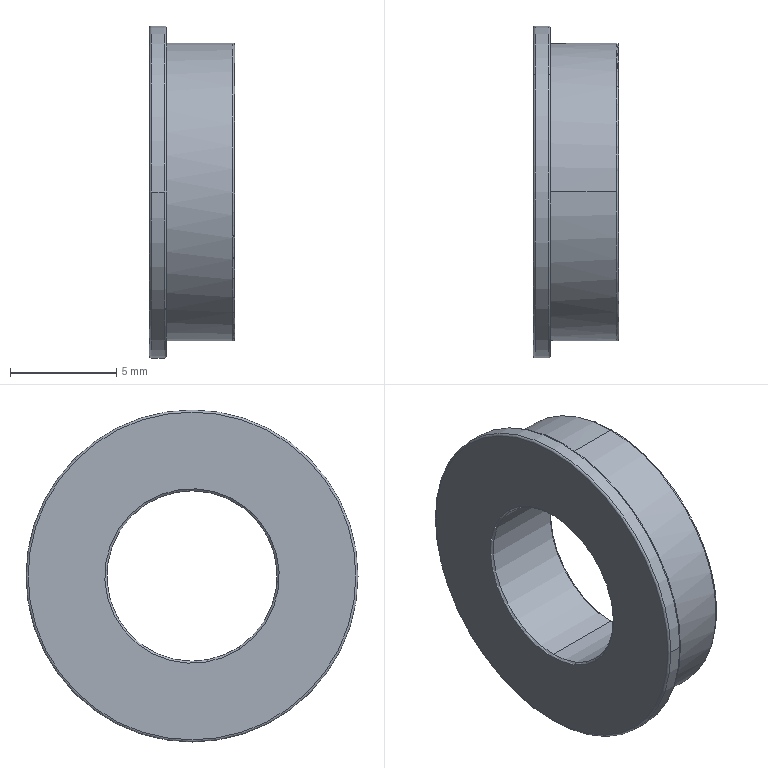Part | STEP file | ASND-0110-0502110051 | 1 solid | 19 faces | box 4 x 15.6 x 15.6 mm | volume 444.035 mm3 | torus 10 | cylinder 6 | plane 3 | commonest cylinder face diameters 8 x2 14 x2 15.6 x2
STEP:
#1=CARTESIAN_POINT('',(0.,0.,0.));
#2=DIRECTION('',(0.,0.,1.));
#3=DIRECTION('',(1.,0.,0.));
#4=AXIS2_PLACEMENT_3D('',#1,#2,#3);
#5=CARTESIAN_POINT('',(0.,-5.445,-5.445));
#6=VERTEX_POINT('',#5);
#7=CARTESIAN_POINT('',(0.,5.445,5.445));
#8=VERTEX_POINT('',#7);
#9=CARTESIAN_POINT('',(0.,0.,0.));
#10=DIRECTION('',(-1.,0.,0.));
#11=DIRECTION('',(0.,1.,0.));
#12=AXIS2_PLACEMENT_3D('',#9,#10,#11);
#13=CIRCLE('',#12,7.7);
#14=CARTESIAN_POINT('',(0.1,0.,0.));
#15=DIRECTION('',(1.,0.,0.));
#16=DIRECTION('',(0.,0.7071,0.7071));
#17=AXIS2_PLACEMENT_3D('',#14,#15,#16);
#18=TOROIDAL_SURFACE('',#17,7.7,0.1);
#19=CARTESIAN_POINT('',(5.498,4.712));
#20=DIRECTION('',(-1.,0.));
#21=VECTOR('',#20,1.);
#22=LINE('',#19,#21);
#23=(GEOMETRIC_REPRESENTATION_CONTEXT(2)PARAMETRIC_REPRESENTATION_CONTEXT()REPRESENTATION_CONTEXT('',''));
#24=DEFINITIONAL_REPRESENTATION('',(#22),#23);
#25=PCURVE('',#18,#24);
#26=CARTESIAN_POINT('',(0.,0.,0.));
#27=DIRECTION('',(1.,0.,0.));
#28=DIRECTION('',(0.,0.7071,0.7071));
#29=AXIS2_PLACEMENT_3D('',#26,#27,#28);
#30=PLANE('',#29);
#31=CARTESIAN_POINT('',(5.445,-5.445));
#32=CARTESIAN_POINT('',(-3.986,-14.875));
#33=CARTESIAN_POINT('',(-7.438,-1.993));
#34=CARTESIAN_POINT('',(-10.889,10.889));
#35=CARTESIAN_POINT('',(1.993,7.438));
#36=CARTESIAN_POINT('',(14.875,3.986));
#37=CARTESIAN_POINT('',(5.445,-5.445));
#38=(BOUNDED_CURVE()B_SPLINE_CURVE(2,(#31,#32,#33,#34,#35,#36,#37),.UNSPECIFIED.,.T.,.F.)B_SPLINE_CURVE_WITH_KNOTS((1,2,2,2,2,1),(-2.094,0.,2.094,4.189,6.283,8.378),.UNSPECIFIED.)CURVE()GEOMETRIC_REPRESENTATION_ITEM()RATIONAL_B_SPLINE_CURVE((1.,0.5,1.,0.5,1.,0.5,1.))REPRESENTATION_ITEM(''));
#39=(GEOMETRIC_REPRESENTATION_CONTEXT(2)PARAMETRIC_REPRESENTATION_CONTEXT()REPRESENTATION_CONTEXT('',''));
#40=DEFINITIONAL_REPRESENTATION('',(#38),#39);
#41=PCURVE('',#30,#40);
#42=SURFACE_CURVE('',#13,(#25,#41),.PCURVE_S1.);
#43=EDGE_CURVE('',#6,#8,#42,.T.);
#44=ORIENTED_EDGE('',*,*,#43,.F.);
#45=CARTESIAN_POINT('',(0.1,-5.515,-5.515));
#46=VERTEX_POINT('',#45);
#47=CARTESIAN_POINT('',(0.1,-5.445,-5.445));
#48=DIRECTION('',(0.,-0.7071,0.7071));
#49=DIRECTION('',(0.,-0.7071,-0.7071));
#50=AXIS2_PLACEMENT_3D('',#47,#48,#49);
#51=CIRCLE('',#50,0.1);
#52=CARTESIAN_POINT('',(3.142,0.));
#53=DIRECTION('',(0.,1.));
#54=VECTOR('',#53,1.);
#55=LINE('',#52,#54);
#56=(GEOMETRIC_REPRESENTATION_CONTEXT(2)PARAMETRIC_REPRESENTATION_CONTEXT()REPRESENTATION_CONTEXT('',''));
#57=DEFINITIONAL_REPRESENTATION('',(#55),#56);
#58=PCURVE('',#18,#57);
#59=CARTESIAN_POINT('',(0.1,0.,0.));
#60=DIRECTION('',(1.,0.,0.));
#61=DIRECTION('',(0.,0.7071,0.7071));
#62=AXIS2_PLACEMENT_3D('',#59,#60,#61);
#63=TOROIDAL_SURFACE('',#62,7.7,0.1);
#64=CARTESIAN_POINT('',(3.142,0.));
#65=DIRECTION('',(0.,1.));
#66=VECTOR('',#65,1.);
#67=LINE('',#64,#66);
#68=(GEOMETRIC_REPRESENTATION_CONTEXT(2)PARAMETRIC_REPRESENTATION_CONTEXT()REPRESENTATION_CONTEXT('',''));
#69=DEFINITIONAL_REPRESENTATION('',(#67),#68);
#70=PCURVE('',#63,#69);
#71=SURFACE_CURVE('',#51,(#58,#70),.PCURVE_S1.);
#72=EDGE_CURVE('',#6,#46,#71,.T.);
#73=ORIENTED_EDGE('',*,*,#72,.T.);
#74=CARTESIAN_POINT('',(0.1,-7.8,0.));
#75=VERTEX_POINT('',#74);
#76=CARTESIAN_POINT('',(0.1,0.,0.));
#77=DIRECTION('',(-1.,0.,0.));
#78=DIRECTION('',(0.,1.,0.));
#79=AXIS2_PLACEMENT_3D('',#76,#77,#78);
#80=CIRCLE('',#79,7.8);
#81=CARTESIAN_POINT('',(5.498,6.283));
#82=DIRECTION('',(-1.,0.));
#83=VECTOR('',#82,1.);
#84=LINE('',#81,#83);
#85=(GEOMETRIC_REPRESENTATION_CONTEXT(2)PARAMETRIC_REPRESENTATION_CONTEXT()REPRESENTATION_CONTEXT('',''));
#86=DEFINITIONAL_REPRESENTATION('',(#84),#85);
#87=PCURVE('',#18,#86);
#88=CARTESIAN_POINT('',(-0.04,0.,0.));
#89=DIRECTION('',(1.,0.,0.));
#90=DIRECTION('',(0.,-1.,0.));
#91=AXIS2_PLACEMENT_3D('',#88,#89,#90);
#92=CYLINDRICAL_SURFACE('',#91,7.8);
#93=CARTESIAN_POINT('',(3.142,0.14));
#94=DIRECTION('',(-1.,0.));
#95=VECTOR('',#94,1.);
#96=LINE('',#93,#95);
#97=(GEOMETRIC_REPRESENTATION_CONTEXT(2)PARAMETRIC_REPRESENTATION_CONTEXT()REPRESENTATION_CONTEXT('',''));
#98=DEFINITIONAL_REPRESENTATION('',(#96),#97);
#99=PCURVE('',#92,#98);
#100=SURFACE_CURVE('',#80,(#87,#99),.PCURVE_S1.);
#101=EDGE_CURVE('',#46,#75,#100,.T.);
#102=ORIENTED_EDGE('',*,*,#101,.T.);
#103=CARTESIAN_POINT('',(0.1,5.515,5.515));
#104=VERTEX_POINT('',#103);
#105=CARTESIAN_POINT('',(0.1,0.,0.));
#106=DIRECTION('',(-1.,0.,0.));
#107=DIRECTION('',(0.,1.,0.));
#108=AXIS2_PLACEMENT_3D('',#105,#106,#107);
#109=CIRCLE('',#108,7.8);
#110=CARTESIAN_POINT('',(5.498,6.283));
#111=DIRECTION('',(-1.,0.));
#112=VECTOR('',#111,1.);
#113=LINE('',#110,#112);
#114=(GEOMETRIC_REPRESENTATION_CONTEXT(2)PARAMETRIC_REPRESENTATION_CONTEXT()REPRESENTATION_CONTEXT('',''));
#115=DEFINITIONAL_REPRESENTATION('',(#113),#114);
#116=PCURVE('',#18,#115);
#117=CARTESIAN_POINT('',(-0.04,0.,0.));
#118=DIRECTION('',(1.,0.,0.));
#119=DIRECTION('',(0.,-1.,0.));
#120=AXIS2_PLACEMENT_3D('',#117,#118,#119);
#121=CYLINDRICAL_SURFACE('',#120,7.8);
#122=CARTESIAN_POINT('',(9.425,0.14));
#123=DIRECTION('',(-1.,0.));
#124=VECTOR('',#123,1.);
#125=LINE('',#122,#124);
#126=(GEOMETRIC_REPRESENTATION_CONTEXT(2)PARAMETRIC_REPRESENTATION_CONTEXT()REPRESENTATION_CONTEXT('',''));
#127=DEFINITIONAL_REPRESENTATION('',(#125),#126);
#128=PCURVE('',#121,#127);
#129=SURFACE_CURVE('',#109,(#116,#128),.PCURVE_S1.);
#130=EDGE_CURVE('',#75,#104,#129,.T.);
#131=ORIENTED_EDGE('',*,*,#130,.T.);
#132=CARTESIAN_POINT('',(0.1,5.445,5.445));
#133=DIRECTION('',(0.,0.7071,-0.7071));
#134=DIRECTION('',(0.,0.7071,0.7071));
#135=AXIS2_PLACEMENT_3D('',#132,#133,#134);
#136=CIRCLE('',#135,0.1);
#137=CARTESIAN_POINT('',(0.,0.));
#138=DIRECTION('',(0.,1.));
#139=VECTOR('',#138,1.);
#140=LINE('',#137,#139);
#141=(GEOMETRIC_REPRESENTATION_CONTEXT(2)PARAMETRIC_REPRESENTATION_CONTEXT()REPRESENTATION_CONTEXT('',''));
#142=DEFINITIONAL_REPRESENTATION('',(#140),#141);
#143=PCURVE('',#18,#142);
#144=CARTESIAN_POINT('',(6.283,0.));
#145=DIRECTION('',(0.,1.));
#146=VECTOR('',#145,1.);
#147=LINE('',#144,#146);
#148=(GEOMETRIC_REPRESENTATION_CONTEXT(2)PARAMETRIC_REPRESENTATION_CONTEXT()REPRESENTATION_CONTEXT('',''));
#149=DEFINITIONAL_REPRESENTATION('',(#147),#148);
#150=PCURVE('',#63,#149);
#151=SURFACE_CURVE('',#136,(#143,#150),.PCURVE_S1.);
#152=EDGE_CURVE('',#8,#104,#151,.T.);
#153=ORIENTED_EDGE('',*,*,#152,.F.);
#154=EDGE_LOOP('',(#44,#73,#102,#131,#153));
#155=FACE_BOUND('',#154,.T.);
#156=ADVANCED_FACE('',(#155),#18,.T.);
#157=CARTESIAN_POINT('',(0.1,7.8,0.));
#158=VERTEX_POINT('',#157);
#159=CARTESIAN_POINT('',(0.1,0.,0.));
#160=DIRECTION('',(-1.,0.,0.));
#161=DIRECTION('',(0.,1.,0.));
#162=AXIS2_PLACEMENT_3D('',#159,#160,#161);
#163=CIRCLE('',#162,7.8);
#164=CARTESIAN_POINT('',(3.142,0.14));
#165=DIRECTION('',(-1.,0.));
#166=VECTOR('',#165,1.);
#167=LINE('',#164,#166);
#168=(GEOMETRIC_REPRESENTATION_CONTEXT(2)PARAMETRIC_REPRESENTATION_CONTEXT()REPRESENTATION_CONTEXT('',''));
#169=DEFINITIONAL_REPRESENTATION('',(#167),#168);
#170=PCURVE('',#92,#169);
#171=CARTESIAN_POINT('',(5.498,6.283));
#172=DIRECTION('',(-1.,0.));
#173=VECTOR('',#172,1.);
#174=LINE('',#171,#173);
#175=(GEOMETRIC_REPRESENTATION_CONTEXT(2)PARAMETRIC_REPRESENTATION_CONTEXT()REPRESENTATION_CONTEXT('',''));
#176=DEFINITIONAL_REPRESENTATION('',(#174),#175);
#177=PCURVE('',#63,#176);
#178=SURFACE_CURVE('',#163,(#170,#177),.PCURVE_S1.);
#179=EDGE_CURVE('',#158,#46,#178,.T.);
#180=ORIENTED_EDGE('',*,*,#179,.F.);
#181=CARTESIAN_POINT('',(0.7,7.8,0.));
#182=VERTEX_POINT('',#181);
#183=CARTESIAN_POINT('',(-0.04,7.8,0.));
#184=DIRECTION('',(1.,0.,0.));
#185=VECTOR('',#184,1.);
#186=LINE('',#183,#185);
#187=CARTESIAN_POINT('',(3.142,0.));
#188=DIRECTION('',(0.,1.));
#189=VECTOR('',#188,1.);
#190=LINE('',#187,#189);
#191=(GEOMETRIC_REPRESENTATION_CONTEXT(2)PARAMETRIC_REPRESENTATION_CONTEXT()REPRESENTATION_CONTEXT('',''));
#192=DEFINITIONAL_REPRESENTATION('',(#190),#191);
#193=PCURVE('',#92,#192);
#194=CARTESIAN_POINT('',(3.142,0.));
#195=DIRECTION('',(0.,1.));
#196=VECTOR('',#195,1.);
#197=LINE('',#194,#196);
#198=(GEOMETRIC_REPRESENTATION_CONTEXT(2)PARAMETRIC_REPRESENTATION_CONTEXT()REPRESENTATION_CONTEXT('',''));
#199=DEFINITIONAL_REPRESENTATION('',(#197),#198);
#200=PCURVE('',#121,#199);
#201=SURFACE_CURVE('',#186,(#193,#200),.PCURVE_S1.);
#202=EDGE_CURVE('',#158,#182,#201,.T.);
#203=ORIENTED_EDGE('',*,*,#202,.T.);
#204=CARTESIAN_POINT('',(0.7,-5.515,-5.515));
#205=VERTEX_POINT('',#204);
#206=CARTESIAN_POINT('',(0.7,0.,0.));
#207=DIRECTION('',(-1.,0.,0.));
#208=DIRECTION('',(0.,1.,0.));
#209=AXIS2_PLACEMENT_3D('',#206,#207,#208);
#210=CIRCLE('',#209,7.8);
#211=CARTESIAN_POINT('',(3.142,0.74));
#212=DIRECTION('',(-1.,0.));
#213=VECTOR('',#212,1.);
#214=LINE('',#211,#213);
#215=(GEOMETRIC_REPRESENTATION_CONTEXT(2)PARAMETRIC_REPRESENTATION_CONTEXT()REPRESENTATION_CONTEXT('',''));
#216=DEFINITIONAL_REPRESENTATION('',(#214),#215);
#217=PCURVE('',#92,#216);
#218=CARTESIAN_POINT('',(0.7,0.,0.));
#219=DIRECTION('',(1.,0.,0.));
#220=DIRECTION('',(0.,0.7071,0.7071));
#221=AXIS2_PLACEMENT_3D('',#218,#219,#220);
#222=TOROIDAL_SURFACE('',#221,7.7,0.1);
#223=CARTESIAN_POINT('',(5.498,0.));
#224=DIRECTION('',(-1.,0.));
#225=VECTOR('',#224,1.);
#226=LINE('',#223,#225);
#227=(GEOMETRIC_REPRESENTATION_CONTEXT(2)PARAMETRIC_REPRESENTATION_CONTEXT()REPRESENTATION_CONTEXT('',''));
#228=DEFINITIONAL_REPRESENTATION('',(#226),#227);
#229=PCURVE('',#222,#228);
#230=SURFACE_CURVE('',#210,(#217,#229),.PCURVE_S1.);
#231=EDGE_CURVE('',#182,#205,#230,.T.);
#232=ORIENTED_EDGE('',*,*,#231,.T.);
#233=CARTESIAN_POINT('',(0.7,-7.8,0.));
#234=VERTEX_POINT('',#233);
#235=CARTESIAN_POINT('',(0.7,0.,0.));
#236=DIRECTION('',(-1.,0.,0.));
#237=DIRECTION('',(0.,1.,0.));
#238=AXIS2_PLACEMENT_3D('',#235,#236,#237);
#239=CIRCLE('',#238,7.8);
#240=CARTESIAN_POINT('',(3.142,0.74));
#241=DIRECTION('',(-1.,0.));
#242=VECTOR('',#241,1.);
#243=LINE('',#240,#242);
#244=(GEOMETRIC_REPRESENTATION_CONTEXT(2)PARAMETRIC_REPRESENTATION_CONTEXT()REPRESENTATION_CONTEXT('',''));
#245=DEFINITIONAL_REPRESENTATION('',(#243),#244);
#246=PCURVE('',#92,#245);
#247=CARTESIAN_POINT('',(0.7,0.,0.));
#248=DIRECTION('',(1.,0.,0.));
#249=DIRECTION('',(0.,0.7071,0.7071));
#250=AXIS2_PLACEMENT_3D('',#247,#248,#249);
#251=TOROIDAL_SURFACE('',#250,7.7,0.1);
#252=CARTESIAN_POINT('',(5.498,0.));
#253=DIRECTION('',(-1.,0.));
#254=VECTOR('',#253,1.);
#255=LINE('',#252,#254);
#256=(GEOMETRIC_REPRESENTATION_CONTEXT(2)PARAMETRIC_REPRESENTATION_CONTEXT()REPRESENTATION_CONTEXT('',''));
#257=DEFINITIONAL_REPRESENTATION('',(#255),#256);
#258=PCURVE('',#251,#257);
#259=SURFACE_CURVE('',#239,(#246,#258),.PCURVE_S1.);
#260=EDGE_CURVE('',#205,#234,#259,.T.);
#261=ORIENTED_EDGE('',*,*,#260,.T.);
#262=CARTESIAN_POINT('',(-0.04,-7.8,0.));
#263=DIRECTION('',(1.,0.,0.));
#264=VECTOR('',#263,1.);
#265=LINE('',#262,#264);
#266=CARTESIAN_POINT('',(0.,0.));
#267=DIRECTION('',(0.,1.));
#268=VECTOR('',#267,1.);
#269=LINE('',#266,#268);
#270=(GEOMETRIC_REPRESENTATION_CONTEXT(2)PARAMETRIC_REPRESENTATION_CONTEXT()REPRESENTATION_CONTEXT('',''));
#271=DEFINITIONAL_REPRESENTATION('',(#269),#270);
#272=PCURVE('',#92,#271);
#273=CARTESIAN_POINT('',(6.283,0.));
#274=DIRECTION('',(0.,1.));
#275=VECTOR('',#274,1.);
#276=LINE('',#273,#275);
#277=(GEOMETRIC_REPRESENTATION_CONTEXT(2)PARAMETRIC_REPRESENTATION_CONTEXT()REPRESENTATION_CONTEXT('',''));
#278=DEFINITIONAL_REPRESENTATION('',(#276),#277);
#279=PCURVE('',#121,#278);
#280=SURFACE_CURVE('',#265,(#272,#279),.PCURVE_S1.);
#281=EDGE_CURVE('',#75,#234,#280,.T.);
#282=ORIENTED_EDGE('',*,*,#281,.F.);
#283=ORIENTED_EDGE('',*,*,#101,.F.);
#284=EDGE_LOOP('',(#180,#203,#232,#261,#282,#283));
#285=FACE_BOUND('',#284,.T.);
#286=ADVANCED_FACE('',(#285),#92,.T.);
#287=ORIENTED_EDGE('',*,*,#260,.F.);
#288=CARTESIAN_POINT('',(0.8,-5.445,-5.445));
#289=VERTEX_POINT('',#288);
#290=CARTESIAN_POINT('',(0.7,-5.445,-5.445));
#291=DIRECTION('',(0.,-0.7071,0.7071));
#292=DIRECTION('',(0.,-0.7071,-0.7071));
#293=AXIS2_PLACEMENT_3D('',#290,#291,#292);
#294=CIRCLE('',#293,0.1);
#295=CARTESIAN_POINT('',(3.142,0.));
#296=DIRECTION('',(0.,1.));
#297=VECTOR('',#296,1.);
#298=LINE('',#295,#297);
#299=(GEOMETRIC_REPRESENTATION_CONTEXT(2)PARAMETRIC_REPRESENTATION_CONTEXT()REPRESENTATION_CONTEXT('',''));
#300=DEFINITIONAL_REPRESENTATION('',(#298),#299);
#301=PCURVE('',#251,#300);
#302=CARTESIAN_POINT('',(3.142,0.));
#303=DIRECTION('',(0.,1.));
#304=VECTOR('',#303,1.);
#305=LINE('',#302,#304);
#306=(GEOMETRIC_REPRESENTATION_CONTEXT(2)PARAMETRIC_REPRESENTATION_CONTEXT()REPRESENTATION_CONTEXT('',''));
#307=DEFINITIONAL_REPRESENTATION('',(#305),#306);
#308=PCURVE('',#222,#307);
#309=SURFACE_CURVE('',#294,(#301,#308),.PCURVE_S1.);
#310=EDGE_CURVE('',#205,#289,#309,.T.);
#311=ORIENTED_EDGE('',*,*,#310,.T.);
#312=CARTESIAN_POINT('',(0.8,5.445,5.445));
#313=VERTEX_POINT('',#312);
#314=CARTESIAN_POINT('',(0.8,0.,0.));
#315=DIRECTION('',(-1.,0.,0.));
#316=DIRECTION('',(0.,1.,0.));
#317=AXIS2_PLACEMENT_3D('',#314,#315,#316);
#318=CIRCLE('',#317,7.7);
#319=CARTESIAN_POINT('',(5.498,1.571));
#320=DIRECTION('',(-1.,0.));
#321=VECTOR('',#320,1.);
#322=LINE('',#319,#321);
#323=(GEOMETRIC_REPRESENTATION_CONTEXT(2)PARAMETRIC_REPRESENTATION_CONTEXT()REPRESENTATION_CONTEXT('',''));
#324=DEFINITIONAL_REPRESENTATION('',(#322),#323);
#325=PCURVE('',#251,#324);
#326=CARTESIAN_POINT('',(0.8,0.,0.));
#327=DIRECTION('',(1.,0.,0.));
#328=DIRECTION('',(0.,0.7071,0.7071));
#329=AXIS2_PLACEMENT_3D('',#326,#327,#328);
#330=PLANE('',#329);
#331=CARTESIAN_POINT('',(5.445,-5.445));
#332=CARTESIAN_POINT('',(-3.986,-14.875));
#333=CARTESIAN_POINT('',(-7.438,-1.993));
#334=CARTESIAN_POINT('',(-10.889,10.889));
#335=CARTESIAN_POINT('',(1.993,7.438));
#336=CARTESIAN_POINT('',(14.875,3.986));
#337=CARTESIAN_POINT('',(5.445,-5.445));
#338=(BOUNDED_CURVE()B_SPLINE_CURVE(2,(#331,#332,#333,#334,#335,#336,#337),.UNSPECIFIED.,.T.,.F.)B_SPLINE_CURVE_WITH_KNOTS((1,2,2,2,2,1),(-2.094,0.,2.094,4.189,6.283,8.378),.UNSPECIFIED.)CURVE()GEOMETRIC_REPRESENTATION_ITEM()RATIONAL_B_SPLINE_CURVE((1.,0.5,1.,0.5,1.,0.5,1.))REPRESENTATION_ITEM(''));
#339=(GEOMETRIC_REPRESENTATION_CONTEXT(2)PARAMETRIC_REPRESENTATION_CONTEXT()REPRESENTATION_CONTEXT('',''));
#340=DEFINITIONAL_REPRESENTATION('',(#338),#339);
#341=PCURVE('',#330,#340);
#342=SURFACE_CURVE('',#318,(#325,#341),.PCURVE_S1.);
#343=EDGE_CURVE('',#289,#313,#342,.T.);
#344=ORIENTED_EDGE('',*,*,#343,.T.);
#345=CARTESIAN_POINT('',(0.7,5.515,5.515));
#346=VERTEX_POINT('',#345);
#347=CARTESIAN_POINT('',(0.7,5.445,5.445));
#348=DIRECTION('',(0.,0.7071,-0.7071));
#349=DIRECTION('',(0.,0.7071,0.7071));
#350=AXIS2_PLACEMENT_3D('',#347,#348,#349);
#351=CIRCLE('',#350,0.1);
#352=CARTESIAN_POINT('',(0.,0.));
#353=DIRECTION('',(0.,1.));
#354=VECTOR('',#353,1.);
#355=LINE('',#352,#354);
#356=(GEOMETRIC_REPRESENTATION_CONTEXT(2)PARAMETRIC_REPRESENTATION_CONTEXT()REPRESENTATION_CONTEXT('',''));
#357=DEFINITIONAL_REPRESENTATION('',(#355),#356);
#358=PCURVE('',#251,#357);
#359=CARTESIAN_POINT('',(6.283,0.));
#360=DIRECTION('',(0.,1.));
#361=VECTOR('',#360,1.);
#362=LINE('',#359,#361);
#363=(GEOMETRIC_REPRESENTATION_CONTEXT(2)PARAMETRIC_REPRESENTATION_CONTEXT()REPRESENTATION_CONTEXT('',''));
#364=DEFINITIONAL_REPRESENTATION('',(#362),#363);
#365=PCURVE('',#222,#364);
#366=SURFACE_CURVE('',#351,(#358,#365),.PCURVE_S1.);
#367=EDGE_CURVE('',#346,#313,#366,.T.);
#368=ORIENTED_EDGE('',*,*,#367,.F.);
#369=CARTESIAN_POINT('',(0.7,0.,0.));
#370=DIRECTION('',(-1.,0.,0.));
#371=DIRECTION('',(0.,1.,0.));
#372=AXIS2_PLACEMENT_3D('',#369,#370,#371);
#373=CIRCLE('',#372,7.8);
#374=CARTESIAN_POINT('',(5.498,0.));
#375=DIRECTION('',(-1.,0.));
#376=VECTOR('',#375,1.);
#377=LINE('',#374,#376);
#378=(GEOMETRIC_REPRESENTATION_CONTEXT(2)PARAMETRIC_REPRESENTATION_CONTEXT()REPRESENTATION_CONTEXT('',''));
#379=DEFINITIONAL_REPRESENTATION('',(#377),#378);
#380=PCURVE('',#251,#379);
#381=CARTESIAN_POINT('',(9.425,0.74));
#382=DIRECTION('',(-1.,0.));
#383=VECTOR('',#382,1.);
#384=LINE('',#381,#383);
#385=(GEOMETRIC_REPRESENTATION_CONTEXT(2)PARAMETRIC_REPRESENTATION_CONTEXT()REPRESENTATION_CONTEXT('',''));
#386=DEFINITIONAL_REPRESENTATION('',(#384),#385);
#387=PCURVE('',#121,#386);
#388=SURFACE_CURVE('',#373,(#380,#387),.PCURVE_S1.);
#389=EDGE_CURVE('',#234,#346,#388,.T.);
#390=ORIENTED_EDGE('',*,*,#389,.F.);
#391=EDGE_LOOP('',(#287,#311,#344,#368,#390));
#392=FACE_BOUND('',#391,.T.);
#393=ADVANCED_FACE('',(#392),#251,.T.);
#394=CARTESIAN_POINT('',(0.8,0.,7.));
#395=VERTEX_POINT('',#394);
#396=CARTESIAN_POINT('',(0.8,0.,-7.));
#397=VERTEX_POINT('',#396);
#398=CARTESIAN_POINT('',(0.8,0.,0.));
#399=DIRECTION('',(1.,0.,0.));
#400=DIRECTION('',(0.,0.,1.));
#401=AXIS2_PLACEMENT_3D('',#398,#399,#400);
#402=CIRCLE('',#401,7.);
#403=CARTESIAN_POINT('',(0.,0.,0.));
#404=DIRECTION('',(1.,0.,0.));
#405=DIRECTION('',(0.,0.,1.));
#406=AXIS2_PLACEMENT_3D('',#403,#404,#405);
#407=CYLINDRICAL_SURFACE('',#406,7.);
#408=CARTESIAN_POINT('',(0.,0.8));
#409=DIRECTION('',(1.,0.));
#410=VECTOR('',#409,1.);
#411=LINE('',#408,#410);
#412=(GEOMETRIC_REPRESENTATION_CONTEXT(2)PARAMETRIC_REPRESENTATION_CONTEXT()REPRESENTATION_CONTEXT('',''));
#413=DEFINITIONAL_REPRESENTATION('',(#411),#412);
#414=PCURVE('',#407,#413);
#415=CARTESIAN_POINT('',(0.,0.));
#416=DIRECTION('',(0.7071,0.7071));
#417=AXIS2_PLACEMENT_2D('',#415,#416);
#418=CIRCLE('',#417,7.);
#419=(GEOMETRIC_REPRESENTATION_CONTEXT(2)PARAMETRIC_REPRESENTATION_CONTEXT()REPRESENTATION_CONTEXT('',''));
#420=DEFINITIONAL_REPRESENTATION('',(#418),#419);
#421=PCURVE('',#330,#420);
#422=SURFACE_CURVE('',#402,(#414,#421),.PCURVE_S1.);
#423=EDGE_CURVE('',#395,#397,#422,.T.);
#424=ORIENTED_EDGE('',*,*,#423,.T.);
#425=CARTESIAN_POINT('',(3.9,0.,-7.));
#426=VERTEX_POINT('',#425);
#427=CARTESIAN_POINT('',(0.,0.,-7.));
#428=DIRECTION('',(1.,0.,0.));
#429=VECTOR('',#428,1.);
#430=LINE('',#427,#429);
#431=CARTESIAN_POINT('',(3.142,0.));
#432=DIRECTION('',(0.,1.));
#433=VECTOR('',#432,1.);
#434=LINE('',#431,#433);
#435=(GEOMETRIC_REPRESENTATION_CONTEXT(2)PARAMETRIC_REPRESENTATION_CONTEXT()REPRESENTATION_CONTEXT('',''));
#436=DEFINITIONAL_REPRESENTATION('',(#434),#435);
#437=PCURVE('',#407,#436);
#438=CARTESIAN_POINT('',(0.,0.,0.));
#439=DIRECTION('',(1.,0.,0.));
#440=DIRECTION('',(0.,0.,1.));
#441=AXIS2_PLACEMENT_3D('',#438,#439,#440);
#442=CYLINDRICAL_SURFACE('',#441,7.);
#443=CARTESIAN_POINT('',(3.142,0.));
#444=DIRECTION('',(0.,1.));
#445=VECTOR('',#444,1.);
#446=LINE('',#443,#445);
#447=(GEOMETRIC_REPRESENTATION_CONTEXT(2)PARAMETRIC_REPRESENTATION_CONTEXT()REPRESENTATION_CONTEXT('',''));
#448=DEFINITIONAL_REPRESENTATION('',(#446),#447);
#449=PCURVE('',#442,#448);
#450=SURFACE_CURVE('',#430,(#437,#449),.PCURVE_S1.);
#451=EDGE_CURVE('',#397,#426,#450,.T.);
#452=ORIENTED_EDGE('',*,*,#451,.T.);
#453=CARTESIAN_POINT('',(3.9,-4.95,-4.95));
#454=VERTEX_POINT('',#453);
#455=CARTESIAN_POINT('',(3.9,0.,0.));
#456=DIRECTION('',(1.,0.,0.));
#457=DIRECTION('',(0.,0.,-1.));
#458=AXIS2_PLACEMENT_3D('',#455,#456,#457);
#459=CIRCLE('',#458,7.);
#460=CARTESIAN_POINT('',(-3.142,3.9));
#461=DIRECTION('',(1.,0.));
#462=VECTOR('',#461,1.);
#463=LINE('',#460,#462);
#464=(GEOMETRIC_REPRESENTATION_CONTEXT(2)PARAMETRIC_REPRESENTATION_CONTEXT()REPRESENTATION_CONTEXT('',''));
#465=DEFINITIONAL_REPRESENTATION('',(#463),#464);
#466=PCURVE('',#407,#465);
#467=CARTESIAN_POINT('',(3.9,0.,0.));
#468=DIRECTION('',(1.,0.,0.));
#469=DIRECTION('',(0.,0.7071,0.7071));
#470=AXIS2_PLACEMENT_3D('',#467,#468,#469);
#471=TOROIDAL_SURFACE('',#470,6.9,0.1);
#472=CARTESIAN_POINT('',(-2.356,0.));
#473=DIRECTION('',(1.,0.));
#474=VECTOR('',#473,1.);
#475=LINE('',#472,#474);
#476=(GEOMETRIC_REPRESENTATION_CONTEXT(2)PARAMETRIC_REPRESENTATION_CONTEXT()REPRESENTATION_CONTEXT('',''));
#477=DEFINITIONAL_REPRESENTATION('',(#475),#476);
#478=PCURVE('',#471,#477);
#479=SURFACE_CURVE('',#459,(#466,#478),.PCURVE_S1.);
#480=EDGE_CURVE('',#454,#426,#479,.T.);
#481=ORIENTED_EDGE('',*,*,#480,.F.);
#482=CARTESIAN_POINT('',(3.9,0.,7.));
#483=VERTEX_POINT('',#482);
#484=CARTESIAN_POINT('',(3.9,0.,0.));
#485=DIRECTION('',(1.,0.,0.));
#486=DIRECTION('',(0.,0.,-1.));
#487=AXIS2_PLACEMENT_3D('',#484,#485,#486);
#488=CIRCLE('',#487,7.);
#489=CARTESIAN_POINT('',(-3.142,3.9));
#490=DIRECTION('',(1.,0.));
#491=VECTOR('',#490,1.);
#492=LINE('',#489,#491);
#493=(GEOMETRIC_REPRESENTATION_CONTEXT(2)PARAMETRIC_REPRESENTATION_CONTEXT()REPRESENTATION_CONTEXT('',''));
#494=DEFINITIONAL_REPRESENTATION('',(#492),#493);
#495=PCURVE('',#407,#494);
#496=CARTESIAN_POINT('',(3.9,0.,0.));
#497=DIRECTION('',(1.,0.,0.));
#498=DIRECTION('',(0.,0.7071,0.7071));
#499=AXIS2_PLACEMENT_3D('',#496,#497,#498);
#500=TOROIDAL_SURFACE('',#499,6.9,0.1);
#501=CARTESIAN_POINT('',(-2.356,0.));
#502=DIRECTION('',(1.,0.));
#503=VECTOR('',#502,1.);
#504=LINE('',#501,#503);
#505=(GEOMETRIC_REPRESENTATION_CONTEXT(2)PARAMETRIC_REPRESENTATION_CONTEXT()REPRESENTATION_CONTEXT('',''));
#506=DEFINITIONAL_REPRESENTATION('',(#504),#505);
#507=PCURVE('',#500,#506);
#508=SURFACE_CURVE('',#488,(#495,#507),.PCURVE_S1.);
#509=EDGE_CURVE('',#483,#454,#508,.T.);
#510=ORIENTED_EDGE('',*,*,#509,.F.);
#511=CARTESIAN_POINT('',(0.,0.,7.));
#512=DIRECTION('',(1.,0.,0.));
#513=VECTOR('',#512,1.);
#514=LINE('',#511,#513);
#515=CARTESIAN_POINT('',(0.,0.));
#516=DIRECTION('',(0.,1.));
#517=VECTOR('',#516,1.);
#518=LINE('',#515,#517);
#519=(GEOMETRIC_REPRESENTATION_CONTEXT(2)PARAMETRIC_REPRESENTATION_CONTEXT()REPRESENTATION_CONTEXT('',''));
#520=DEFINITIONAL_REPRESENTATION('',(#518),#519);
#521=PCURVE('',#407,#520);
#522=CARTESIAN_POINT('',(6.283,0.));
#523=DIRECTION('',(0.,1.));
#524=VECTOR('',#523,1.);
#525=LINE('',#522,#524);
#526=(GEOMETRIC_REPRESENTATION_CONTEXT(2)PARAMETRIC_REPRESENTATION_CONTEXT()REPRESENTATION_CONTEXT('',''));
#527=DEFINITIONAL_REPRESENTATION('',(#525),#526);
#528=PCURVE('',#442,#527);
#529=SURFACE_CURVE('',#514,(#521,#528),.PCURVE_S1.);
#530=EDGE_CURVE('',#395,#483,#529,.T.);
#531=ORIENTED_EDGE('',*,*,#530,.F.);
#532=EDGE_LOOP('',(#424,#452,#481,#510,#531));
#533=FACE_BOUND('',#532,.T.);
#534=ADVANCED_FACE('',(#533),#407,.T.);
#535=CARTESIAN_POINT('',(3.9,4.95,4.95));
#536=VERTEX_POINT('',#535);
#537=CARTESIAN_POINT('',(4.,4.879,4.879));
#538=VERTEX_POINT('',#537);
#539=CARTESIAN_POINT('',(3.9,4.879,4.879));
#540=DIRECTION('',(0.,0.7071,-0.7071));
#541=DIRECTION('',(0.,0.7071,0.7071));
#542=AXIS2_PLACEMENT_3D('',#539,#540,#541);
#543=CIRCLE('',#542,0.1);
#544=CARTESIAN_POINT('',(0.,0.));
#545=DIRECTION('',(0.,1.));
#546=VECTOR('',#545,1.);
#547=LINE('',#544,#546);
#548=(GEOMETRIC_REPRESENTATION_CONTEXT(2)PARAMETRIC_REPRESENTATION_CONTEXT()REPRESENTATION_CONTEXT('',''));
#549=DEFINITIONAL_REPRESENTATION('',(#547),#548);
#550=PCURVE('',#500,#549);
#551=CARTESIAN_POINT('',(6.283,0.));
#552=DIRECTION('',(0.,1.));
#553=VECTOR('',#552,1.);
#554=LINE('',#551,#553);
#555=(GEOMETRIC_REPRESENTATION_CONTEXT(2)PARAMETRIC_REPRESENTATION_CONTEXT()REPRESENTATION_CONTEXT('',''));
#556=DEFINITIONAL_REPRESENTATION('',(#554),#555);
#557=PCURVE('',#471,#556);
#558=SURFACE_CURVE('',#543,(#550,#557),.PCURVE_S1.);
#559=EDGE_CURVE('',#536,#538,#558,.T.);
#560=ORIENTED_EDGE('',*,*,#559,.F.);
#561=CARTESIAN_POINT('',(3.9,0.,0.));
#562=DIRECTION('',(1.,0.,0.));
#563=DIRECTION('',(0.,0.,-1.));
#564=AXIS2_PLACEMENT_3D('',#561,#562,#563);
#565=CIRCLE('',#564,7.);
#566=CARTESIAN_POINT('',(-2.356,0.));
#567=DIRECTION('',(1.,0.));
#568=VECTOR('',#567,1.);
#569=LINE('',#566,#568);
#570=(GEOMETRIC_REPRESENTATION_CONTEXT(2)PARAMETRIC_REPRESENTATION_CONTEXT()REPRESENTATION_CONTEXT('',''));
#571=DEFINITIONAL_REPRESENTATION('',(#569),#570);
#572=PCURVE('',#500,#571);
#573=CARTESIAN_POINT('',(3.142,3.9));
#574=DIRECTION('',(1.,0.));
#575=VECTOR('',#574,1.);
#576=LINE('',#573,#575);
#577=(GEOMETRIC_REPRESENTATION_CONTEXT(2)PARAMETRIC_REPRESENTATION_CONTEXT()REPRESENTATION_CONTEXT('',''));
#578=DEFINITIONAL_REPRESENTATION('',(#576),#577);
#579=PCURVE('',#442,#578);
#580=SURFACE_CURVE('',#565,(#572,#579),.PCURVE_S1.);
#581=EDGE_CURVE('',#536,#483,#580,.T.);
#582=ORIENTED_EDGE('',*,*,#581,.T.);
#583=ORIENTED_EDGE('',*,*,#509,.T.);
#584=CARTESIAN_POINT('',(4.,-4.879,-4.879));
#585=VERTEX_POINT('',#584);
#586=CARTESIAN_POINT('',(3.9,-4.879,-4.879));
#587=DIRECTION('',(0.,-0.7071,0.7071));
#588=DIRECTION('',(0.,-0.7071,-0.7071));
#589=AXIS2_PLACEMENT_3D('',#586,#587,#588);
#590=CIRCLE('',#589,0.1);
#591=CARTESIAN_POINT('',(3.142,0.));
#592=DIRECTION('',(0.,1.));
#593=VECTOR('',#592,1.);
#594=LINE('',#591,#593);
#595=(GEOMETRIC_REPRESENTATION_CONTEXT(2)PARAMETRIC_REPRESENTATION_CONTEXT()REPRESENTATION_CONTEXT('',''));
#596=DEFINITIONAL_REPRESENTATION('',(#594),#595);
#597=PCURVE('',#500,#596);
#598=CARTESIAN_POINT('',(3.142,0.));
#599=DIRECTION('',(0.,1.));
#600=VECTOR('',#599,1.);
#601=LINE('',#598,#600);
#602=(GEOMETRIC_REPRESENTATION_CONTEXT(2)PARAMETRIC_REPRESENTATION_CONTEXT()REPRESENTATION_CONTEXT('',''));
#603=DEFINITIONAL_REPRESENTATION('',(#601),#602);
#604=PCURVE('',#471,#603);
#605=SURFACE_CURVE('',#590,(#597,#604),.PCURVE_S1.);
#606=EDGE_CURVE('',#454,#585,#605,.T.);
#607=ORIENTED_EDGE('',*,*,#606,.T.);
#608=CARTESIAN_POINT('',(4.,0.,0.));
#609=DIRECTION('',(1.,0.,0.));
#610=DIRECTION('',(0.,0.,-1.));
#611=AXIS2_PLACEMENT_3D('',#608,#609,#610);
#612=CIRCLE('',#611,6.9);
#613=CARTESIAN_POINT('',(-2.356,1.571));
#614=DIRECTION('',(1.,0.));
#615=VECTOR('',#614,1.);
#616=LINE('',#613,#615);
#617=(GEOMETRIC_REPRESENTATION_CONTEXT(2)PARAMETRIC_REPRESENTATION_CONTEXT()REPRESENTATION_CONTEXT('',''));
#618=DEFINITIONAL_REPRESENTATION('',(#616),#617);
#619=PCURVE('',#500,#618);
#620=CARTESIAN_POINT('',(4.,0.,0.));
#621=DIRECTION('',(1.,0.,0.));
#622=DIRECTION('',(0.,0.7071,0.7071));
#623=AXIS2_PLACEMENT_3D('',#620,#621,#622);
#624=PLANE('',#623);
#625=CARTESIAN_POINT('',(0.,0.));
#626=DIRECTION('',(-0.7071,-0.7071));
#627=AXIS2_PLACEMENT_2D('',#625,#626);
#628=CIRCLE('',#627,6.9);
#629=(GEOMETRIC_REPRESENTATION_CONTEXT(2)PARAMETRIC_REPRESENTATION_CONTEXT()REPRESENTATION_CONTEXT('',''));
#630=DEFINITIONAL_REPRESENTATION('',(#628),#629);
#631=PCURVE('',#624,#630);
#632=SURFACE_CURVE('',#612,(#619,#631),.PCURVE_S1.);
#633=EDGE_CURVE('',#538,#585,#632,.T.);
#634=ORIENTED_EDGE('',*,*,#633,.F.);
#635=EDGE_LOOP('',(#560,#582,#583,#607,#634));
#636=FACE_BOUND('',#635,.T.);
#637=ADVANCED_FACE('',(#636),#500,.T.);
#638=CARTESIAN_POINT('',(4.,-2.899,-2.899));
#639=VERTEX_POINT('',#638);
#640=CARTESIAN_POINT('',(4.,2.899,2.899));
#641=VERTEX_POINT('',#640);
#642=CARTESIAN_POINT('',(4.,0.,0.));
#643=DIRECTION('',(-1.,0.,0.));
#644=DIRECTION('',(0.,0.,1.));
#645=AXIS2_PLACEMENT_3D('',#642,#643,#644);
#646=CIRCLE('',#645,4.1);
#647=CARTESIAN_POINT('',(3.9,0.,0.));
#648=DIRECTION('',(1.,0.,0.));
#649=DIRECTION('',(0.,0.7071,0.7071));
#650=AXIS2_PLACEMENT_3D('',#647,#648,#649);
#651=TOROIDAL_SURFACE('',#650,4.1,0.1);
#652=CARTESIAN_POINT('',(7.069,1.571));
#653=DIRECTION('',(-1.,0.));
#654=VECTOR('',#653,1.);
#655=LINE('',#652,#654);
#656=(GEOMETRIC_REPRESENTATION_CONTEXT(2)PARAMETRIC_REPRESENTATION_CONTEXT()REPRESENTATION_CONTEXT('',''));
#657=DEFINITIONAL_REPRESENTATION('',(#655),#656);
#658=PCURVE('',#651,#657);
#659=CARTESIAN_POINT('',(2.899,2.899));
#660=CARTESIAN_POINT('',(7.921,-2.122));
#661=CARTESIAN_POINT('',(1.061,-3.96));
#662=CARTESIAN_POINT('',(-5.798,-5.798));
#663=CARTESIAN_POINT('',(-3.96,1.061));
#664=CARTESIAN_POINT('',(-2.122,7.921));
#665=CARTESIAN_POINT('',(2.899,2.899));
#666=(BOUNDED_CURVE()B_SPLINE_CURVE(2,(#659,#660,#661,#662,#663,#664,#665),.UNSPECIFIED.,.T.,.F.)B_SPLINE_CURVE_WITH_KNOTS((1,2,2,2,2,1),(-2.094,0.,2.094,4.189,6.283,8.378),.UNSPECIFIED.)CURVE()GEOMETRIC_REPRESENTATION_ITEM()RATIONAL_B_SPLINE_CURVE((1.,0.5,1.,0.5,1.,0.5,1.))REPRESENTATION_ITEM(''));
#667=(GEOMETRIC_REPRESENTATION_CONTEXT(2)PARAMETRIC_REPRESENTATION_CONTEXT()REPRESENTATION_CONTEXT('',''));
#668=DEFINITIONAL_REPRESENTATION('',(#666),#667);
#669=PCURVE('',#624,#668);
#670=SURFACE_CURVE('',#646,(#658,#669),.PCURVE_S1.);
#671=EDGE_CURVE('',#639,#641,#670,.T.);
#672=ORIENTED_EDGE('',*,*,#671,.F.);
#673=CARTESIAN_POINT('',(3.9,-2.828,-2.828));
#674=VERTEX_POINT('',#673);
#675=CARTESIAN_POINT('',(3.9,-2.899,-2.899));
#676=DIRECTION('',(0.,-0.7071,0.7071));
#677=DIRECTION('',(0.,-0.7071,-0.7071));
#678=AXIS2_PLACEMENT_3D('',#675,#676,#677);
#679=CIRCLE('',#678,0.1);
#680=CARTESIAN_POINT('',(3.142,0.));
#681=DIRECTION('',(0.,1.));
#682=VECTOR('',#681,1.);
#683=LINE('',#680,#682);
#684=(GEOMETRIC_REPRESENTATION_CONTEXT(2)PARAMETRIC_REPRESENTATION_CONTEXT()REPRESENTATION_CONTEXT('',''));
#685=DEFINITIONAL_REPRESENTATION('',(#683),#684);
#686=PCURVE('',#651,#685);
#687=CARTESIAN_POINT('',(3.9,0.,0.));
#688=DIRECTION('',(1.,0.,0.));
#689=DIRECTION('',(0.,0.7071,0.7071));
#690=AXIS2_PLACEMENT_3D('',#687,#688,#689);
#691=TOROIDAL_SURFACE('',#690,4.1,0.1);
#692=CARTESIAN_POINT('',(3.142,0.));
#693=DIRECTION('',(0.,1.));
#694=VECTOR('',#693,1.);
#695=LINE('',#692,#694);
#696=(GEOMETRIC_REPRESENTATION_CONTEXT(2)PARAMETRIC_REPRESENTATION_CONTEXT()REPRESENTATION_CONTEXT('',''));
#697=DEFINITIONAL_REPRESENTATION('',(#695),#696);
#698=PCURVE('',#691,#697);
#699=SURFACE_CURVE('',#679,(#686,#698),.PCURVE_S1.);
#700=EDGE_CURVE('',#639,#674,#699,.T.);
#701=ORIENTED_EDGE('',*,*,#700,.T.);
#702=CARTESIAN_POINT('',(3.9,0.,4.));
#703=VERTEX_POINT('',#702);
#704=CARTESIAN_POINT('',(3.9,0.,0.));
#705=DIRECTION('',(-1.,0.,0.));
#706=DIRECTION('',(0.,0.,-1.));
#707=AXIS2_PLACEMENT_3D('',#704,#705,#706);
#708=CIRCLE('',#707,4.);
#709=CARTESIAN_POINT('',(3.927,3.142));
#710=DIRECTION('',(-1.,0.));
#711=VECTOR('',#710,1.);
#712=LINE('',#709,#711);
#713=(GEOMETRIC_REPRESENTATION_CONTEXT(2)PARAMETRIC_REPRESENTATION_CONTEXT()REPRESENTATION_CONTEXT('',''));
#714=DEFINITIONAL_REPRESENTATION('',(#712),#713);
#715=PCURVE('',#651,#714);
#716=CARTESIAN_POINT('',(0.,0.,0.));
#717=DIRECTION('',(1.,0.,0.));
#718=DIRECTION('',(0.,0.,1.));
#719=AXIS2_PLACEMENT_3D('',#716,#717,#718);
#720=CYLINDRICAL_SURFACE('',#719,4.);
#721=CARTESIAN_POINT('',(3.142,3.9));
#722=DIRECTION('',(-1.,0.));
#723=VECTOR('',#722,1.);
#724=LINE('',#721,#723);
#725=(GEOMETRIC_REPRESENTATION_CONTEXT(2)PARAMETRIC_REPRESENTATION_CONTEXT()REPRESENTATION_CONTEXT('',''));
#726=DEFINITIONAL_REPRESENTATION('',(#724),#725);
#727=PCURVE('',#720,#726);
#728=SURFACE_CURVE('',#708,(#715,#727),.PCURVE_S1.);
#729=EDGE_CURVE('',#674,#703,#728,.T.);
#730=ORIENTED_EDGE('',*,*,#729,.T.);
#731=CARTESIAN_POINT('',(3.9,2.828,2.828));
#732=VERTEX_POINT('',#731);
#733=CARTESIAN_POINT('',(3.9,0.,0.));
#734=DIRECTION('',(-1.,0.,0.));
#735=DIRECTION('',(0.,0.,-1.));
#736=AXIS2_PLACEMENT_3D('',#733,#734,#735);
#737=CIRCLE('',#736,4.);
#738=CARTESIAN_POINT('',(3.927,3.142));
#739=DIRECTION('',(-1.,0.));
#740=VECTOR('',#739,1.);
#741=LINE('',#738,#740);
#742=(GEOMETRIC_REPRESENTATION_CONTEXT(2)PARAMETRIC_REPRESENTATION_CONTEXT()REPRESENTATION_CONTEXT('',''));
#743=DEFINITIONAL_REPRESENTATION('',(#741),#742);
#744=PCURVE('',#651,#743);
#745=CARTESIAN_POINT('',(0.,0.,0.));
#746=DIRECTION('',(1.,0.,0.));
#747=DIRECTION('',(0.,0.,1.));
#748=AXIS2_PLACEMENT_3D('',#745,#746,#747);
#749=CYLINDRICAL_SURFACE('',#748,4.);
#750=CARTESIAN_POINT('',(9.425,3.9));
#751=DIRECTION('',(-1.,0.));
#752=VECTOR('',#751,1.);
#753=LINE('',#750,#752);
#754=(GEOMETRIC_REPRESENTATION_CONTEXT(2)PARAMETRIC_REPRESENTATION_CONTEXT()REPRESENTATION_CONTEXT('',''));
#755=DEFINITIONAL_REPRESENTATION('',(#753),#754);
#756=PCURVE('',#749,#755);
#757=SURFACE_CURVE('',#737,(#744,#756),.PCURVE_S1.);
#758=EDGE_CURVE('',#703,#732,#757,.T.);
#759=ORIENTED_EDGE('',*,*,#758,.T.);
#760=CARTESIAN_POINT('',(3.9,2.899,2.899));
#761=DIRECTION('',(0.,0.7071,-0.7071));
#762=DIRECTION('',(0.,0.7071,0.7071));
#763=AXIS2_PLACEMENT_3D('',#760,#761,#762);
#764=CIRCLE('',#763,0.1);
#765=CARTESIAN_POINT('',(0.,0.));
#766=DIRECTION('',(0.,1.));
#767=VECTOR('',#766,1.);
#768=LINE('',#765,#767);
#769=(GEOMETRIC_REPRESENTATION_CONTEXT(2)PARAMETRIC_REPRESENTATION_CONTEXT()REPRESENTATION_CONTEXT('',''));
#770=DEFINITIONAL_REPRESENTATION('',(#768),#769);
#771=PCURVE('',#651,#770);
#772=CARTESIAN_POINT('',(6.283,0.));
#773=DIRECTION('',(0.,1.));
#774=VECTOR('',#773,1.);
#775=LINE('',#772,#774);
#776=(GEOMETRIC_REPRESENTATION_CONTEXT(2)PARAMETRIC_REPRESENTATION_CONTEXT()REPRESENTATION_CONTEXT('',''));
#777=DEFINITIONAL_REPRESENTATION('',(#775),#776);
#778=PCURVE('',#691,#777);
#779=SURFACE_CURVE('',#764,(#771,#778),.PCURVE_S1.);
#780=EDGE_CURVE('',#641,#732,#779,.T.);
#781=ORIENTED_EDGE('',*,*,#780,.F.);
#782=EDGE_LOOP('',(#672,#701,#730,#759,#781));
#783=FACE_BOUND('',#782,.T.);
#784=ADVANCED_FACE('',(#783),#651,.T.);
#785=CARTESIAN_POINT('',(0.1,2.828,2.828));
#786=VERTEX_POINT('',#785);
#787=CARTESIAN_POINT('',(0.1,0.,4.));
#788=VERTEX_POINT('',#787);
#789=CARTESIAN_POINT('',(0.1,0.,0.));
#790=DIRECTION('',(1.,0.,0.));
#791=DIRECTION('',(0.,0.,-1.));
#792=AXIS2_PLACEMENT_3D('',#789,#790,#791);
#793=CIRCLE('',#792,4.);
#794=CARTESIAN_POINT('',(3.142,0.1));
#795=DIRECTION('',(1.,0.));
#796=VECTOR('',#795,1.);
#797=LINE('',#794,#796);
#798=(GEOMETRIC_REPRESENTATION_CONTEXT(2)PARAMETRIC_REPRESENTATION_CONTEXT()REPRESENTATION_CONTEXT('',''));
#799=DEFINITIONAL_REPRESENTATION('',(#797),#798);
#800=PCURVE('',#749,#799);
#801=CARTESIAN_POINT('',(0.1,0.,0.));
#802=DIRECTION('',(1.,0.,0.));
#803=DIRECTION('',(0.,0.7071,0.7071));
#804=AXIS2_PLACEMENT_3D('',#801,#802,#803);
#805=TOROIDAL_SURFACE('',#804,4.1,0.1);
#806=CARTESIAN_POINT('',(-2.356,3.142));
#807=DIRECTION('',(1.,0.));
#808=VECTOR('',#807,1.);
#809=LINE('',#806,#808);
#810=(GEOMETRIC_REPRESENTATION_CONTEXT(2)PARAMETRIC_REPRESENTATION_CONTEXT()REPRESENTATION_CONTEXT('',''));
#811=DEFINITIONAL_REPRESENTATION('',(#809),#810);
#812=PCURVE('',#805,#811);
#813=SURFACE_CURVE('',#793,(#800,#812),.PCURVE_S1.);
#814=EDGE_CURVE('',#786,#788,#813,.T.);
#815=ORIENTED_EDGE('',*,*,#814,.T.);
#816=CARTESIAN_POINT('',(0.,0.,4.));
#817=DIRECTION('',(1.,0.,0.));
#818=VECTOR('',#817,1.);
#819=LINE('',#816,#818);
#820=CARTESIAN_POINT('',(6.283,0.));
#821=DIRECTION('',(0.,1.));
#822=VECTOR('',#821,1.);
#823=LINE('',#820,#822);
#824=(GEOMETRIC_REPRESENTATION_CONTEXT(2)PARAMETRIC_REPRESENTATION_CONTEXT()REPRESENTATION_CONTEXT('',''));
#825=DEFINITIONAL_REPRESENTATION('',(#823),#824);
#826=PCURVE('',#749,#825);
#827=CARTESIAN_POINT('',(0.,0.));
#828=DIRECTION('',(0.,1.));
#829=VECTOR('',#828,1.);
#830=LINE('',#827,#829);
#831=(GEOMETRIC_REPRESENTATION_CONTEXT(2)PARAMETRIC_REPRESENTATION_CONTEXT()REPRESENTATION_CONTEXT('',''));
#832=DEFINITIONAL_REPRESENTATION('',(#830),#831);
#833=PCURVE('',#720,#832);
#834=SURFACE_CURVE('',#819,(#826,#833),.PCURVE_S1.);
#835=EDGE_CURVE('',#788,#703,#834,.T.);
#836=ORIENTED_EDGE('',*,*,#835,.T.);
#837=ORIENTED_EDGE('',*,*,#758,.T.);
#838=CARTESIAN_POINT('',(3.9,0.,-4.));
#839=VERTEX_POINT('',#838);
#840=CARTESIAN_POINT('',(3.9,0.,0.));
#841=DIRECTION('',(-1.,0.,0.));
#842=DIRECTION('',(0.,0.,-1.));
#843=AXIS2_PLACEMENT_3D('',#840,#841,#842);
#844=CIRCLE('',#843,4.);
#845=CARTESIAN_POINT('',(9.425,3.9));
#846=DIRECTION('',(-1.,0.));
#847=VECTOR('',#846,1.);
#848=LINE('',#845,#847);
#849=(GEOMETRIC_REPRESENTATION_CONTEXT(2)PARAMETRIC_REPRESENTATION_CONTEXT()REPRESENTATION_CONTEXT('',''));
#850=DEFINITIONAL_REPRESENTATION('',(#848),#849);
#851=PCURVE('',#749,#850);
#852=CARTESIAN_POINT('',(10.21,3.142));
#853=DIRECTION('',(-1.,0.));
#854=VECTOR('',#853,1.);
#855=LINE('',#852,#854);
#856=(GEOMETRIC_REPRESENTATION_CONTEXT(2)PARAMETRIC_REPRESENTATION_CONTEXT()REPRESENTATION_CONTEXT('',''));
#857=DEFINITIONAL_REPRESENTATION('',(#855),#856);
#858=PCURVE('',#691,#857);
#859=SURFACE_CURVE('',#844,(#851,#858),.PCURVE_S1.);
#860=EDGE_CURVE('',#732,#839,#859,.T.);
#861=ORIENTED_EDGE('',*,*,#860,.T.);
#862=CARTESIAN_POINT('',(0.1,0.,-4.));
#863=VERTEX_POINT('',#862);
#864=CARTESIAN_POINT('',(0.,0.,-4.));
#865=DIRECTION('',(1.,0.,0.));
#866=VECTOR('',#865,1.);
#867=LINE('',#864,#866);
#868=CARTESIAN_POINT('',(3.142,0.));
#869=DIRECTION('',(0.,1.));
#870=VECTOR('',#869,1.);
#871=LINE('',#868,#870);
#872=(GEOMETRIC_REPRESENTATION_CONTEXT(2)PARAMETRIC_REPRESENTATION_CONTEXT()REPRESENTATION_CONTEXT('',''));
#873=DEFINITIONAL_REPRESENTATION('',(#871),#872);
#874=PCURVE('',#749,#873);
#875=CARTESIAN_POINT('',(3.142,0.));
#876=DIRECTION('',(0.,1.));
#877=VECTOR('',#876,1.);
#878=LINE('',#875,#877);
#879=(GEOMETRIC_REPRESENTATION_CONTEXT(2)PARAMETRIC_REPRESENTATION_CONTEXT()REPRESENTATION_CONTEXT('',''));
#880=DEFINITIONAL_REPRESENTATION('',(#878),#879);
#881=PCURVE('',#720,#880);
#882=SURFACE_CURVE('',#867,(#874,#881),.PCURVE_S1.);
#883=EDGE_CURVE('',#863,#839,#882,.T.);
#884=ORIENTED_EDGE('',*,*,#883,.F.);
#885=CARTESIAN_POINT('',(0.1,0.,0.));
#886=DIRECTION('',(1.,0.,0.));
#887=DIRECTION('',(0.,0.,-1.));
#888=AXIS2_PLACEMENT_3D('',#885,#886,#887);
#889=CIRCLE('',#888,4.);
#890=CARTESIAN_POINT('',(3.142,0.1));
#891=DIRECTION('',(1.,0.));
#892=VECTOR('',#891,1.);
#893=LINE('',#890,#892);
#894=(GEOMETRIC_REPRESENTATION_CONTEXT(2)PARAMETRIC_REPRESENTATION_CONTEXT()REPRESENTATION_CONTEXT('',''));
#895=DEFINITIONAL_REPRESENTATION('',(#893),#894);
#896=PCURVE('',#749,#895);
#897=CARTESIAN_POINT('',(0.1,0.,0.));
#898=DIRECTION('',(1.,0.,0.));
#899=DIRECTION('',(0.,0.7071,0.7071));
#900=AXIS2_PLACEMENT_3D('',#897,#898,#899);
#901=TOROIDAL_SURFACE('',#900,4.1,0.1);
#902=CARTESIAN_POINT('',(3.927,3.142));
#903=DIRECTION('',(1.,0.));
#904=VECTOR('',#903,1.);
#905=LINE('',#902,#904);
#906=(GEOMETRIC_REPRESENTATION_CONTEXT(2)PARAMETRIC_REPRESENTATION_CONTEXT()REPRESENTATION_CONTEXT('',''));
#907=DEFINITIONAL_REPRESENTATION('',(#905),#906);
#908=PCURVE('',#901,#907);
#909=SURFACE_CURVE('',#889,(#896,#908),.PCURVE_S1.);
#910=EDGE_CURVE('',#863,#786,#909,.T.);
#911=ORIENTED_EDGE('',*,*,#910,.T.);
#912=EDGE_LOOP('',(#815,#836,#837,#861,#884,#911));
#913=FACE_BOUND('',#912,.F.);
#914=ADVANCED_FACE('',(#913),#749,.F.);
#915=CARTESIAN_POINT('',(0.,2.899,2.899));
#916=VERTEX_POINT('',#915);
#917=CARTESIAN_POINT('',(0.1,2.899,2.899));
#918=DIRECTION('',(0.,0.7071,-0.7071));
#919=DIRECTION('',(0.,0.7071,0.7071));
#920=AXIS2_PLACEMENT_3D('',#917,#918,#919);
#921=CIRCLE('',#920,0.1);
#922=CARTESIAN_POINT('',(0.,0.));
#923=DIRECTION('',(0.,1.));
#924=VECTOR('',#923,1.);
#925=LINE('',#922,#924);
#926=(GEOMETRIC_REPRESENTATION_CONTEXT(2)PARAMETRIC_REPRESENTATION_CONTEXT()REPRESENTATION_CONTEXT('',''));
#927=DEFINITIONAL_REPRESENTATION('',(#925),#926);
#928=PCURVE('',#805,#927);
#929=CARTESIAN_POINT('',(6.283,0.));
#930=DIRECTION('',(0.,1.));
#931=VECTOR('',#930,1.);
#932=LINE('',#929,#931);
#933=(GEOMETRIC_REPRESENTATION_CONTEXT(2)PARAMETRIC_REPRESENTATION_CONTEXT()REPRESENTATION_CONTEXT('',''));
#934=DEFINITIONAL_REPRESENTATION('',(#932),#933);
#935=PCURVE('',#901,#934);
#936=SURFACE_CURVE('',#921,(#928,#935),.PCURVE_S1.);
#937=EDGE_CURVE('',#786,#916,#936,.T.);
#938=ORIENTED_EDGE('',*,*,#937,.F.);
#939=ORIENTED_EDGE('',*,*,#814,.T.);
#940=CARTESIAN_POINT('',(0.1,-2.828,-2.828));
#941=VERTEX_POINT('',#940);
#942=CARTESIAN_POINT('',(0.1,0.,0.));
#943=DIRECTION('',(1.,0.,0.));
#944=DIRECTION('',(0.,0.,-1.));
#945=AXIS2_PLACEMENT_3D('',#942,#943,#944);
#946=CIRCLE('',#945,4.);
#947=CARTESIAN_POINT('',(-2.356,3.142));
#948=DIRECTION('',(1.,0.));
#949=VECTOR('',#948,1.);
#950=LINE('',#947,#949);
#951=(GEOMETRIC_REPRESENTATION_CONTEXT(2)PARAMETRIC_REPRESENTATION_CONTEXT()REPRESENTATION_CONTEXT('',''));
#952=DEFINITIONAL_REPRESENTATION('',(#950),#951);
#953=PCURVE('',#805,#952);
#954=CARTESIAN_POINT('',(-3.142,0.1));
#955=DIRECTION('',(1.,0.));
#956=VECTOR('',#955,1.);
#957=LINE('',#954,#956);
#958=(GEOMETRIC_REPRESENTATION_CONTEXT(2)PARAMETRIC_REPRESENTATION_CONTEXT()REPRESENTATION_CONTEXT('',''));
#959=DEFINITIONAL_REPRESENTATION('',(#957),#958);
#960=PCURVE('',#720,#959);
#961=SURFACE_CURVE('',#946,(#953,#960),.PCURVE_S1.);
#962=EDGE_CURVE('',#788,#941,#961,.T.);
#963=ORIENTED_EDGE('',*,*,#962,.T.);
#964=CARTESIAN_POINT('',(0.,-2.899,-2.899));
#965=VERTEX_POINT('',#964);
#966=CARTESIAN_POINT('',(0.1,-2.899,-2.899));
#967=DIRECTION('',(0.,-0.7071,0.7071));
#968=DIRECTION('',(0.,-0.7071,-0.7071));
#969=AXIS2_PLACEMENT_3D('',#966,#967,#968);
#970=CIRCLE('',#969,0.1);
#971=CARTESIAN_POINT('',(3.142,0.));
#972=DIRECTION('',(0.,1.));
#973=VECTOR('',#972,1.);
#974=LINE('',#971,#973);
#975=(GEOMETRIC_REPRESENTATION_CONTEXT(2)PARAMETRIC_REPRESENTATION_CONTEXT()REPRESENTATION_CONTEXT('',''));
#976=DEFINITIONAL_REPRESENTATION('',(#974),#975);
#977=PCURVE('',#805,#976);
#978=CARTESIAN_POINT('',(3.142,0.));
#979=DIRECTION('',(0.,1.));
#980=VECTOR('',#979,1.);
#981=LINE('',#978,#980);
#982=(GEOMETRIC_REPRESENTATION_CONTEXT(2)PARAMETRIC_REPRESENTATION_CONTEXT()REPRESENTATION_CONTEXT('',''));
#983=DEFINITIONAL_REPRESENTATION('',(#981),#982);
#984=PCURVE('',#901,#983);
#985=SURFACE_CURVE('',#970,(#977,#984),.PCURVE_S1.);
#986=EDGE_CURVE('',#941,#965,#985,.T.);
#987=ORIENTED_EDGE('',*,*,#986,.T.);
#988=CARTESIAN_POINT('',(0.,0.,0.));
#989=DIRECTION('',(1.,0.,0.));
#990=DIRECTION('',(0.,0.,-1.));
#991=AXIS2_PLACEMENT_3D('',#988,#989,#990);
#992=CIRCLE('',#991,4.1);
#993=CARTESIAN_POINT('',(-2.356,4.712));
#994=DIRECTION('',(1.,0.));
#995=VECTOR('',#994,1.);
#996=LINE('',#993,#995);
#997=(GEOMETRIC_REPRESENTATION_CONTEXT(2)PARAMETRIC_REPRESENTATION_CONTEXT()REPRESENTATION_CONTEXT('',''));
#998=DEFINITIONAL_REPRESENTATION('',(#996),#997);
#999=PCURVE('',#805,#998);
#1000=CARTESIAN_POINT('',(0.,0.));
#1001=DIRECTION('',(-0.7071,-0.7071));
#1002=AXIS2_PLACEMENT_2D('',#1000,#1001);
#1003=CIRCLE('',#1002,4.1);
#1004=(GEOMETRIC_REPRESENTATION_CONTEXT(2)PARAMETRIC_REPRESENTATION_CONTEXT()REPRESENTATION_CONTEXT('',''));
#1005=DEFINITIONAL_REPRESENTATION('',(#1003),#1004);
#1006=PCURVE('',#30,#1005);
#1007=SURFACE_CURVE('',#992,(#999,#1006),.PCURVE_S1.);
#1008=EDGE_CURVE('',#916,#965,#1007,.T.);
#1009=ORIENTED_EDGE('',*,*,#1008,.F.);
#1010=EDGE_LOOP('',(#938,#939,#963,#987,#1009));
#1011=FACE_BOUND('',#1010,.T.);
#1012=ADVANCED_FACE('',(#1011),#805,.T.);
#1013=CARTESIAN_POINT('',(0.,0.,0.));
#1014=DIRECTION('',(-1.,0.,0.));
#1015=DIRECTION('',(0.,1.,0.));
#1016=AXIS2_PLACEMENT_3D('',#1013,#1014,#1015);
#1017=CIRCLE('',#1016,7.7);
#1018=CARTESIAN_POINT('',(5.445,-5.445));
#1019=CARTESIAN_POINT('',(-3.986,-14.875));
#1020=CARTESIAN_POINT('',(-7.438,-1.993));
#1021=CARTESIAN_POINT('',(-10.889,10.889));
#1022=CARTESIAN_POINT('',(1.993,7.438));
#1023=CARTESIAN_POINT('',(14.875,3.986));
#1024=CARTESIAN_POINT('',(5.445,-5.445));
#1025=(BOUNDED_CURVE()B_SPLINE_CURVE(2,(#1018,#1019,#1020,#1021,#1022,#1023,#1024),.UNSPECIFIED.,.T.,.F.)B_SPLINE_CURVE_WITH_KNOTS((1,2,2,2,2,1),(-2.094,0.,2.094,4.189,6.283,8.378),.UNSPECIFIED.)CURVE()GEOMETRIC_REPRESENTATION_ITEM()RATIONAL_B_SPLINE_CURVE((1.,0.5,1.,0.5,1.,0.5,1.))REPRESENTATION_ITEM(''));
#1026=(GEOMETRIC_REPRESENTATION_CONTEXT(2)PARAMETRIC_REPRESENTATION_CONTEXT()REPRESENTATION_CONTEXT('',''));
#1027=DEFINITIONAL_REPRESENTATION('',(#1025),#1026);
#1028=PCURVE('',#30,#1027);
#1029=CARTESIAN_POINT('',(11.781,4.712));
#1030=DIRECTION('',(-1.,0.));
#1031=VECTOR('',#1030,1.);
#1032=LINE('',#1029,#1031);
#1033=(GEOMETRIC_REPRESENTATION_CONTEXT(2)PARAMETRIC_REPRESENTATION_CONTEXT()REPRESENTATION_CONTEXT('',''));
#1034=DEFINITIONAL_REPRESENTATION('',(#1032),#1033);
#1035=PCURVE('',#63,#1034);
#1036=SURFACE_CURVE('',#1017,(#1028,#1035),.PCURVE_S1.);
#1037=EDGE_CURVE('',#8,#6,#1036,.T.);
#1038=ORIENTED_EDGE('',*,*,#1037,.T.);
#1039=ORIENTED_EDGE('',*,*,#43,.T.);
#1040=EDGE_LOOP('',(#1038,#1039));
#1041=FACE_BOUND('',#1040,.T.);
#1042=ORIENTED_EDGE('',*,*,#1008,.T.);
#1043=CARTESIAN_POINT('',(0.,0.,0.));
#1044=DIRECTION('',(1.,0.,0.));
#1045=DIRECTION('',(0.,0.,-1.));
#1046=AXIS2_PLACEMENT_3D('',#1043,#1044,#1045);
#1047=CIRCLE('',#1046,4.1);
#1048=CARTESIAN_POINT('',(0.,0.));
#1049=DIRECTION('',(-0.7071,-0.7071));
#1050=AXIS2_PLACEMENT_2D('',#1048,#1049);
#1051=CIRCLE('',#1050,4.1);
#1052=(GEOMETRIC_REPRESENTATION_CONTEXT(2)PARAMETRIC_REPRESENTATION_CONTEXT()REPRESENTATION_CONTEXT('',''));
#1053=DEFINITIONAL_REPRESENTATION('',(#1051),#1052);
#1054=PCURVE('',#30,#1053);
#1055=CARTESIAN_POINT('',(-2.356,4.712));
#1056=DIRECTION('',(1.,0.));
#1057=VECTOR('',#1056,1.);
#1058=LINE('',#1055,#1057);
#1059=(GEOMETRIC_REPRESENTATION_CONTEXT(2)PARAMETRIC_REPRESENTATION_CONTEXT()REPRESENTATION_CONTEXT('',''));
#1060=DEFINITIONAL_REPRESENTATION('',(#1058),#1059);
#1061=PCURVE('',#901,#1060);
#1062=SURFACE_CURVE('',#1047,(#1054,#1061),.PCURVE_S1.);
#1063=EDGE_CURVE('',#965,#916,#1062,.T.);
#1064=ORIENTED_EDGE('',*,*,#1063,.T.);
#1065=EDGE_LOOP('',(#1042,#1064));
#1066=FACE_BOUND('',#1065,.T.);
#1067=ADVANCED_FACE('',(#1041,#1066),#30,.F.);
#1068=ORIENTED_EDGE('',*,*,#986,.F.);
#1069=CARTESIAN_POINT('',(0.1,0.,0.));
#1070=DIRECTION('',(1.,0.,0.));
#1071=DIRECTION('',(0.,0.,-1.));
#1072=AXIS2_PLACEMENT_3D('',#1069,#1070,#1071);
#1073=CIRCLE('',#1072,4.);
#1074=CARTESIAN_POINT('',(-2.356,3.142));
#1075=DIRECTION('',(1.,0.));
#1076=VECTOR('',#1075,1.);
#1077=LINE('',#1074,#1076);
#1078=(GEOMETRIC_REPRESENTATION_CONTEXT(2)PARAMETRIC_REPRESENTATION_CONTEXT()REPRESENTATION_CONTEXT('',''));
#1079=DEFINITIONAL_REPRESENTATION('',(#1077),#1078);
#1080=PCURVE('',#901,#1079);
#1081=CARTESIAN_POINT('',(-3.142,0.1));
#1082=DIRECTION('',(1.,0.));
#1083=VECTOR('',#1082,1.);
#1084=LINE('',#1081,#1083);
#1085=(GEOMETRIC_REPRESENTATION_CONTEXT(2)PARAMETRIC_REPRESENTATION_CONTEXT()REPRESENTATION_CONTEXT('',''));
#1086=DEFINITIONAL_REPRESENTATION('',(#1084),#1085);
#1087=PCURVE('',#720,#1086);
#1088=SURFACE_CURVE('',#1073,(#1080,#1087),.PCURVE_S1.);
#1089=EDGE_CURVE('',#941,#863,#1088,.T.);
#1090=ORIENTED_EDGE('',*,*,#1089,.T.);
#1091=ORIENTED_EDGE('',*,*,#910,.T.);
#1092=ORIENTED_EDGE('',*,*,#937,.T.);
#1093=ORIENTED_EDGE('',*,*,#1063,.F.);
#1094=EDGE_LOOP('',(#1068,#1090,#1091,#1092,#1093));
#1095=FACE_BOUND('',#1094,.T.);
#1096=ADVANCED_FACE('',(#1095),#901,.T.);
#1097=CARTESIAN_POINT('',(3.9,0.,0.));
#1098=DIRECTION('',(-1.,0.,0.));
#1099=DIRECTION('',(0.,0.,-1.));
#1100=AXIS2_PLACEMENT_3D('',#1097,#1098,#1099);
#1101=CIRCLE('',#1100,4.);
#1102=CARTESIAN_POINT('',(3.142,3.9));
#1103=DIRECTION('',(-1.,0.));
#1104=VECTOR('',#1103,1.);
#1105=LINE('',#1102,#1104);
#1106=(GEOMETRIC_REPRESENTATION_CONTEXT(2)PARAMETRIC_REPRESENTATION_CONTEXT()REPRESENTATION_CONTEXT('',''));
#1107=DEFINITIONAL_REPRESENTATION('',(#1105),#1106);
#1108=PCURVE('',#720,#1107);
#1109=CARTESIAN_POINT('',(3.927,3.142));
#1110=DIRECTION('',(-1.,0.));
#1111=VECTOR('',#1110,1.);
#1112=LINE('',#1109,#1111);
#1113=(GEOMETRIC_REPRESENTATION_CONTEXT(2)PARAMETRIC_REPRESENTATION_CONTEXT()REPRESENTATION_CONTEXT('',''));
#1114=DEFINITIONAL_REPRESENTATION('',(#1112),#1113);
#1115=PCURVE('',#691,#1114);
#1116=SURFACE_CURVE('',#1101,(#1108,#1115),.PCURVE_S1.);
#1117=EDGE_CURVE('',#839,#674,#1116,.T.);
#1118=ORIENTED_EDGE('',*,*,#1117,.T.);
#1119=ORIENTED_EDGE('',*,*,#729,.T.);
#1120=ORIENTED_EDGE('',*,*,#835,.F.);
#1121=ORIENTED_EDGE('',*,*,#962,.T.);
#1122=ORIENTED_EDGE('',*,*,#1089,.T.);
#1123=ORIENTED_EDGE('',*,*,#883,.T.);
#1124=EDGE_LOOP('',(#1118,#1119,#1120,#1121,#1122,#1123));
#1125=FACE_BOUND('',#1124,.F.);
#1126=ADVANCED_FACE('',(#1125),#720,.F.);
#1127=ORIENTED_EDGE('',*,*,#780,.T.);
#1128=ORIENTED_EDGE('',*,*,#860,.T.);
#1129=ORIENTED_EDGE('',*,*,#1117,.T.);
#1130=ORIENTED_EDGE('',*,*,#700,.F.);
#1131=CARTESIAN_POINT('',(4.,0.,0.));
#1132=DIRECTION('',(-1.,0.,0.));
#1133=DIRECTION('',(0.,0.,1.));
#1134=AXIS2_PLACEMENT_3D('',#1131,#1132,#1133);
#1135=CIRCLE('',#1134,4.1);
#1136=CARTESIAN_POINT('',(7.069,1.571));
#1137=DIRECTION('',(-1.,0.));
#1138=VECTOR('',#1137,1.);
#1139=LINE('',#1136,#1138);
#1140=(GEOMETRIC_REPRESENTATION_CONTEXT(2)PARAMETRIC_REPRESENTATION_CONTEXT()REPRESENTATION_CONTEXT('',''));
#1141=DEFINITIONAL_REPRESENTATION('',(#1139),#1140);
#1142=PCURVE('',#691,#1141);
#1143=CARTESIAN_POINT('',(2.899,2.899));
#1144=CARTESIAN_POINT('',(7.921,-2.122));
#1145=CARTESIAN_POINT('',(1.061,-3.96));
#1146=CARTESIAN_POINT('',(-5.798,-5.798));
#1147=CARTESIAN_POINT('',(-3.96,1.061));
#1148=CARTESIAN_POINT('',(-2.122,7.921));
#1149=CARTESIAN_POINT('',(2.899,2.899));
#1150=(BOUNDED_CURVE()B_SPLINE_CURVE(2,(#1143,#1144,#1145,#1146,#1147,#1148,#1149),.UNSPECIFIED.,.T.,.F.)B_SPLINE_CURVE_WITH_KNOTS((1,2,2,2,2,1),(-2.094,0.,2.094,4.189,6.283,8.378),.UNSPECIFIED.)CURVE()GEOMETRIC_REPRESENTATION_ITEM()RATIONAL_B_SPLINE_CURVE((1.,0.5,1.,0.5,1.,0.5,1.))REPRESENTATION_ITEM(''));
#1151=(GEOMETRIC_REPRESENTATION_CONTEXT(2)PARAMETRIC_REPRESENTATION_CONTEXT()REPRESENTATION_CONTEXT('',''));
#1152=DEFINITIONAL_REPRESENTATION('',(#1150),#1151);
#1153=PCURVE('',#624,#1152);
#1154=SURFACE_CURVE('',#1135,(#1142,#1153),.PCURVE_S1.);
#1155=EDGE_CURVE('',#641,#639,#1154,.T.);
#1156=ORIENTED_EDGE('',*,*,#1155,.F.);
#1157=EDGE_LOOP('',(#1127,#1128,#1129,#1130,#1156));
#1158=FACE_BOUND('',#1157,.T.);
#1159=ADVANCED_FACE('',(#1158),#691,.T.);
#1160=ORIENTED_EDGE('',*,*,#633,.T.);
#1161=CARTESIAN_POINT('',(4.,0.,0.));
#1162=DIRECTION('',(1.,0.,0.));
#1163=DIRECTION('',(0.,0.,-1.));
#1164=AXIS2_PLACEMENT_3D('',#1161,#1162,#1163);
#1165=CIRCLE('',#1164,6.9);
#1166=CARTESIAN_POINT('',(0.,0.));
#1167=DIRECTION('',(-0.7071,-0.7071));
#1168=AXIS2_PLACEMENT_2D('',#1166,#1167);
#1169=CIRCLE('',#1168,6.9);
#1170=(GEOMETRIC_REPRESENTATION_CONTEXT(2)PARAMETRIC_REPRESENTATION_CONTEXT()REPRESENTATION_CONTEXT('',''));
#1171=DEFINITIONAL_REPRESENTATION('',(#1169),#1170);
#1172=PCURVE('',#624,#1171);
#1173=CARTESIAN_POINT('',(-2.356,1.571));
#1174=DIRECTION('',(1.,0.));
#1175=VECTOR('',#1174,1.);
#1176=LINE('',#1173,#1175);
#1177=(GEOMETRIC_REPRESENTATION_CONTEXT(2)PARAMETRIC_REPRESENTATION_CONTEXT()REPRESENTATION_CONTEXT('',''));
#1178=DEFINITIONAL_REPRESENTATION('',(#1176),#1177);
#1179=PCURVE('',#471,#1178);
#1180=SURFACE_CURVE('',#1165,(#1172,#1179),.PCURVE_S1.);
#1181=EDGE_CURVE('',#585,#538,#1180,.T.);
#1182=ORIENTED_EDGE('',*,*,#1181,.T.);
#1183=EDGE_LOOP('',(#1160,#1182));
#1184=FACE_BOUND('',#1183,.T.);
#1185=ORIENTED_EDGE('',*,*,#1155,.T.);
#1186=ORIENTED_EDGE('',*,*,#671,.T.);
#1187=EDGE_LOOP('',(#1185,#1186));
#1188=FACE_BOUND('',#1187,.T.);
#1189=ADVANCED_FACE('',(#1184,#1188),#624,.T.);
#1190=ORIENTED_EDGE('',*,*,#606,.F.);
#1191=ORIENTED_EDGE('',*,*,#480,.T.);
#1192=CARTESIAN_POINT('',(3.9,0.,0.));
#1193=DIRECTION('',(1.,0.,0.));
#1194=DIRECTION('',(0.,0.,-1.));
#1195=AXIS2_PLACEMENT_3D('',#1192,#1193,#1194);
#1196=CIRCLE('',#1195,7.);
#1197=CARTESIAN_POINT('',(3.927,0.));
#1198=DIRECTION('',(1.,0.));
#1199=VECTOR('',#1198,1.);
#1200=LINE('',#1197,#1199);
#1201=(GEOMETRIC_REPRESENTATION_CONTEXT(2)PARAMETRIC_REPRESENTATION_CONTEXT()REPRESENTATION_CONTEXT('',''));
#1202=DEFINITIONAL_REPRESENTATION('',(#1200),#1201);
#1203=PCURVE('',#471,#1202);
#1204=CARTESIAN_POINT('',(3.142,3.9));
#1205=DIRECTION('',(1.,0.));
#1206=VECTOR('',#1205,1.);
#1207=LINE('',#1204,#1206);
#1208=(GEOMETRIC_REPRESENTATION_CONTEXT(2)PARAMETRIC_REPRESENTATION_CONTEXT()REPRESENTATION_CONTEXT('',''));
#1209=DEFINITIONAL_REPRESENTATION('',(#1207),#1208);
#1210=PCURVE('',#442,#1209);
#1211=SURFACE_CURVE('',#1196,(#1203,#1210),.PCURVE_S1.);
#1212=EDGE_CURVE('',#426,#536,#1211,.T.);
#1213=ORIENTED_EDGE('',*,*,#1212,.T.);
#1214=ORIENTED_EDGE('',*,*,#559,.T.);
#1215=ORIENTED_EDGE('',*,*,#1181,.F.);
#1216=EDGE_LOOP('',(#1190,#1191,#1213,#1214,#1215));
#1217=FACE_BOUND('',#1216,.T.);
#1218=ADVANCED_FACE('',(#1217),#471,.T.);
#1219=ORIENTED_EDGE('',*,*,#451,.F.);
#1220=CARTESIAN_POINT('',(0.8,0.,0.));
#1221=DIRECTION('',(1.,0.,0.));
#1222=DIRECTION('',(0.,0.,1.));
#1223=AXIS2_PLACEMENT_3D('',#1220,#1221,#1222);
#1224=CIRCLE('',#1223,7.);
#1225=CARTESIAN_POINT('',(0.,0.8));
#1226=DIRECTION('',(1.,0.));
#1227=VECTOR('',#1226,1.);
#1228=LINE('',#1225,#1227);
#1229=(GEOMETRIC_REPRESENTATION_CONTEXT(2)PARAMETRIC_REPRESENTATION_CONTEXT()REPRESENTATION_CONTEXT('',''));
#1230=DEFINITIONAL_REPRESENTATION('',(#1228),#1229);
#1231=PCURVE('',#442,#1230);
#1232=CARTESIAN_POINT('',(0.,0.));
#1233=DIRECTION('',(0.7071,0.7071));
#1234=AXIS2_PLACEMENT_2D('',#1232,#1233);
#1235=CIRCLE('',#1234,7.);
#1236=(GEOMETRIC_REPRESENTATION_CONTEXT(2)PARAMETRIC_REPRESENTATION_CONTEXT()REPRESENTATION_CONTEXT('',''));
#1237=DEFINITIONAL_REPRESENTATION('',(#1235),#1236);
#1238=PCURVE('',#330,#1237);
#1239=SURFACE_CURVE('',#1224,(#1231,#1238),.PCURVE_S1.);
#1240=EDGE_CURVE('',#397,#395,#1239,.T.);
#1241=ORIENTED_EDGE('',*,*,#1240,.T.);
#1242=ORIENTED_EDGE('',*,*,#530,.T.);
#1243=ORIENTED_EDGE('',*,*,#581,.F.);
#1244=ORIENTED_EDGE('',*,*,#1212,.F.);
#1245=EDGE_LOOP('',(#1219,#1241,#1242,#1243,#1244));
#1246=FACE_BOUND('',#1245,.T.);
#1247=ADVANCED_FACE('',(#1246),#442,.T.);
#1248=CARTESIAN_POINT('',(0.8,0.,0.));
#1249=DIRECTION('',(-1.,0.,0.));
#1250=DIRECTION('',(0.,1.,0.));
#1251=AXIS2_PLACEMENT_3D('',#1248,#1249,#1250);
#1252=CIRCLE('',#1251,7.7);
#1253=CARTESIAN_POINT('',(5.445,-5.445));
#1254=CARTESIAN_POINT('',(-3.986,-14.875));
#1255=CARTESIAN_POINT('',(-7.438,-1.993));
#1256=CARTESIAN_POINT('',(-10.889,10.889));
#1257=CARTESIAN_POINT('',(1.993,7.438));
#1258=CARTESIAN_POINT('',(14.875,3.986));
#1259=CARTESIAN_POINT('',(5.445,-5.445));
#1260=(BOUNDED_CURVE()B_SPLINE_CURVE(2,(#1253,#1254,#1255,#1256,#1257,#1258,#1259),.UNSPECIFIED.,.T.,.F.)B_SPLINE_CURVE_WITH_KNOTS((1,2,2,2,2,1),(-2.094,0.,2.094,4.189,6.283,8.378),.UNSPECIFIED.)CURVE()GEOMETRIC_REPRESENTATION_ITEM()RATIONAL_B_SPLINE_CURVE((1.,0.5,1.,0.5,1.,0.5,1.))REPRESENTATION_ITEM(''));
#1261=(GEOMETRIC_REPRESENTATION_CONTEXT(2)PARAMETRIC_REPRESENTATION_CONTEXT()REPRESENTATION_CONTEXT('',''));
#1262=DEFINITIONAL_REPRESENTATION('',(#1260),#1261);
#1263=PCURVE('',#330,#1262);
#1264=CARTESIAN_POINT('',(11.781,1.571));
#1265=DIRECTION('',(-1.,0.));
#1266=VECTOR('',#1265,1.);
#1267=LINE('',#1264,#1266);
#1268=(GEOMETRIC_REPRESENTATION_CONTEXT(2)PARAMETRIC_REPRESENTATION_CONTEXT()REPRESENTATION_CONTEXT('',''));
#1269=DEFINITIONAL_REPRESENTATION('',(#1267),#1268);
#1270=PCURVE('',#222,#1269);
#1271=SURFACE_CURVE('',#1252,(#1263,#1270),.PCURVE_S1.);
#1272=EDGE_CURVE('',#313,#289,#1271,.T.);
#1273=ORIENTED_EDGE('',*,*,#1272,.F.);
#1274=ORIENTED_EDGE('',*,*,#343,.F.);
#1275=EDGE_LOOP('',(#1273,#1274));
#1276=FACE_BOUND('',#1275,.T.);
#1277=ORIENTED_EDGE('',*,*,#423,.F.);
#1278=ORIENTED_EDGE('',*,*,#1240,.F.);
#1279=EDGE_LOOP('',(#1277,#1278));
#1280=FACE_BOUND('',#1279,.T.);
#1281=ADVANCED_FACE('',(#1276,#1280),#330,.T.);
#1282=ORIENTED_EDGE('',*,*,#310,.F.);
#1283=ORIENTED_EDGE('',*,*,#231,.F.);
#1284=CARTESIAN_POINT('',(0.7,0.,0.));
#1285=DIRECTION('',(-1.,0.,0.));
#1286=DIRECTION('',(0.,1.,0.));
#1287=AXIS2_PLACEMENT_3D('',#1284,#1285,#1286);
#1288=CIRCLE('',#1287,7.8);
#1289=CARTESIAN_POINT('',(11.781,0.));
#1290=DIRECTION('',(-1.,0.));
#1291=VECTOR('',#1290,1.);
#1292=LINE('',#1289,#1291);
#1293=(GEOMETRIC_REPRESENTATION_CONTEXT(2)PARAMETRIC_REPRESENTATION_CONTEXT()REPRESENTATION_CONTEXT('',''));
#1294=DEFINITIONAL_REPRESENTATION('',(#1292),#1293);
#1295=PCURVE('',#222,#1294);
#1296=CARTESIAN_POINT('',(9.425,0.74));
#1297=DIRECTION('',(-1.,0.));
#1298=VECTOR('',#1297,1.);
#1299=LINE('',#1296,#1298);
#1300=(GEOMETRIC_REPRESENTATION_CONTEXT(2)PARAMETRIC_REPRESENTATION_CONTEXT()REPRESENTATION_CONTEXT('',''));
#1301=DEFINITIONAL_REPRESENTATION('',(#1299),#1300);
#1302=PCURVE('',#121,#1301);
#1303=SURFACE_CURVE('',#1288,(#1295,#1302),.PCURVE_S1.);
#1304=EDGE_CURVE('',#346,#182,#1303,.T.);
#1305=ORIENTED_EDGE('',*,*,#1304,.F.);
#1306=ORIENTED_EDGE('',*,*,#367,.T.);
#1307=ORIENTED_EDGE('',*,*,#1272,.T.);
#1308=EDGE_LOOP('',(#1282,#1283,#1305,#1306,#1307));
#1309=FACE_BOUND('',#1308,.T.);
#1310=ADVANCED_FACE('',(#1309),#222,.T.);
#1311=ORIENTED_EDGE('',*,*,#202,.F.);
#1312=CARTESIAN_POINT('',(0.1,0.,0.));
#1313=DIRECTION('',(-1.,0.,0.));
#1314=DIRECTION('',(0.,1.,0.));
#1315=AXIS2_PLACEMENT_3D('',#1312,#1313,#1314);
#1316=CIRCLE('',#1315,7.8);
#1317=CARTESIAN_POINT('',(9.425,0.14));
#1318=DIRECTION('',(-1.,0.));
#1319=VECTOR('',#1318,1.);
#1320=LINE('',#1317,#1319);
#1321=(GEOMETRIC_REPRESENTATION_CONTEXT(2)PARAMETRIC_REPRESENTATION_CONTEXT()REPRESENTATION_CONTEXT('',''));
#1322=DEFINITIONAL_REPRESENTATION('',(#1320),#1321);
#1323=PCURVE('',#121,#1322);
#1324=CARTESIAN_POINT('',(11.781,6.283));
#1325=DIRECTION('',(-1.,0.));
#1326=VECTOR('',#1325,1.);
#1327=LINE('',#1324,#1326);
#1328=(GEOMETRIC_REPRESENTATION_CONTEXT(2)PARAMETRIC_REPRESENTATION_CONTEXT()REPRESENTATION_CONTEXT('',''));
#1329=DEFINITIONAL_REPRESENTATION('',(#1327),#1328);
#1330=PCURVE('',#63,#1329);
#1331=SURFACE_CURVE('',#1316,(#1323,#1330),.PCURVE_S1.);
#1332=EDGE_CURVE('',#104,#158,#1331,.T.);
#1333=ORIENTED_EDGE('',*,*,#1332,.F.);
#1334=ORIENTED_EDGE('',*,*,#130,.F.);
#1335=ORIENTED_EDGE('',*,*,#281,.T.);
#1336=ORIENTED_EDGE('',*,*,#389,.T.);
#1337=ORIENTED_EDGE('',*,*,#1304,.T.);
#1338=EDGE_LOOP('',(#1311,#1333,#1334,#1335,#1336,#1337));
#1339=FACE_BOUND('',#1338,.T.);
#1340=ADVANCED_FACE('',(#1339),#121,.T.);
#1341=ORIENTED_EDGE('',*,*,#72,.F.);
#1342=ORIENTED_EDGE('',*,*,#1037,.F.);
#1343=ORIENTED_EDGE('',*,*,#152,.T.);
#1344=ORIENTED_EDGE('',*,*,#1332,.T.);
#1345=ORIENTED_EDGE('',*,*,#179,.T.);
#1346=EDGE_LOOP('',(#1341,#1342,#1343,#1344,#1345));
#1347=FACE_BOUND('',#1346,.T.);
#1348=ADVANCED_FACE('',(#1347),#63,.T.);
#1349=CLOSED_SHELL('',(#156,#286,#393,#534,#637,#784,#914,#1012,#1067,#1096,#1126,#1159,#1189,#1218,#1247,#1281,#1310,#1340,#1348));
#1350=MANIFOLD_SOLID_BREP('',#1349);
#1351=(LENGTH_UNIT()NAMED_UNIT(*)SI_UNIT(.MILLI.,.METRE.));
#1352=UNCERTAINTY_MEASURE_WITH_UNIT(LENGTH_MEASURE(0.0000001),#1351,'','');
#1353=(NAMED_UNIT(*)PLANE_ANGLE_UNIT()SI_UNIT($,.RADIAN.));
#1354=(NAMED_UNIT(*)SI_UNIT($,.STERADIAN.)SOLID_ANGLE_UNIT());
#1355=(GEOMETRIC_REPRESENTATION_CONTEXT(3)GLOBAL_UNCERTAINTY_ASSIGNED_CONTEXT((#1352))GLOBAL_UNIT_ASSIGNED_CONTEXT((#1351,#1353,#1354))REPRESENTATION_CONTEXT('',''));
#1356=ADVANCED_BREP_SHAPE_REPRESENTATION('',(#4,#1350),#1355);